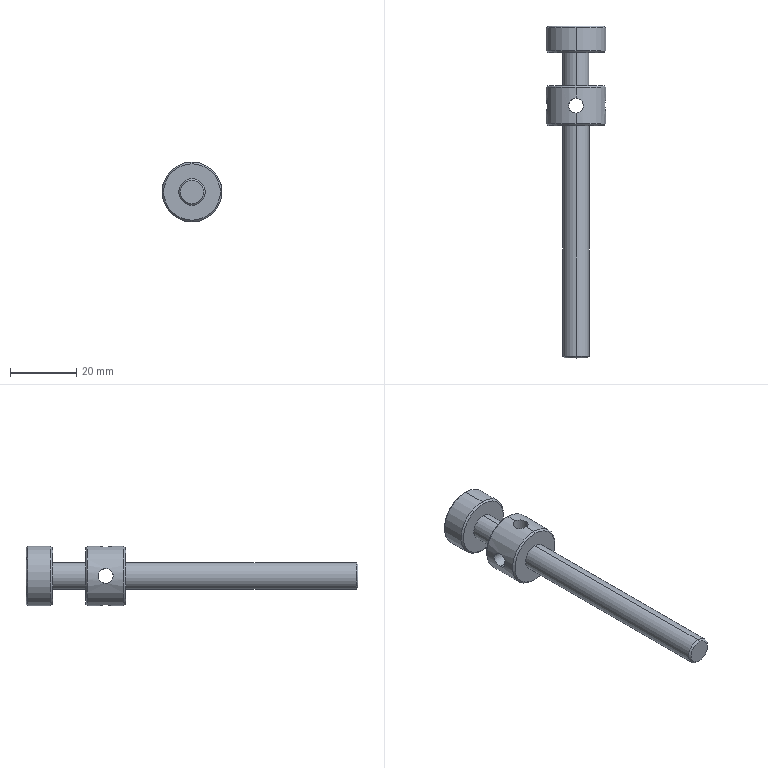Part | SolidWorks | features ICE 4, Chamfer 2, CirPattern 1, Extrusion 1 | 1 solid | 31 faces | box 18 x 100 x 18 mm | volume 8573 mm3 | cylinder 16 | cone 10 | plane 5 | commonest cylinder face diameters 4.5 x8 8 x4 18 x4
STEP:
#1=CARTESIAN_POINT('',(0.,10.,-8.5));
#2=VERTEX_POINT('',#1);
#3=CARTESIAN_POINT('',(0.,10.,8.5));
#4=VERTEX_POINT('',#3);
#5=CARTESIAN_POINT('',(0.,10.,0.));
#6=DIRECTION('',(0.,-1.,0.));
#7=DIRECTION('',(0.,0.,1.));
#8=AXIS2_PLACEMENT_3D('',#5,#6,#7);
#9=CIRCLE('',#8,8.5);
#10=EDGE_CURVE('',#2,#4,#9,.T.);
#11=ORIENTED_EDGE('',*,*,#10,.F.);
#12=CARTESIAN_POINT('',(0.,10.5,-9.));
#13=VERTEX_POINT('',#12);
#14=CARTESIAN_POINT('',(0.,10.5,-9.));
#15=DIRECTION('',(0.,0.7071,-0.7071));
#16=VECTOR('',#15,1000.);
#17=LINE('',#14,#16);
#18=EDGE_CURVE('',#2,#13,#17,.T.);
#19=ORIENTED_EDGE('',*,*,#18,.T.);
#20=CARTESIAN_POINT('',(0.,10.5,9.));
#21=VERTEX_POINT('',#20);
#22=CARTESIAN_POINT('',(0.,10.5,0.));
#23=DIRECTION('',(0.,1.,0.));
#24=DIRECTION('',(0.,0.,1.));
#25=AXIS2_PLACEMENT_3D('',#22,#23,#24);
#26=CIRCLE('',#25,9.);
#27=EDGE_CURVE('',#21,#13,#26,.T.);
#28=ORIENTED_EDGE('',*,*,#27,.F.);
#29=CARTESIAN_POINT('',(0.,10.5,9.));
#30=DIRECTION('',(0.,0.7071,0.7071));
#31=VECTOR('',#30,1000.);
#32=LINE('',#29,#31);
#33=EDGE_CURVE('',#4,#21,#32,.T.);
#34=ORIENTED_EDGE('',*,*,#33,.F.);
#35=EDGE_LOOP('',(#11,#19,#28,#34));
#36=FACE_OUTER_BOUND('',#35,.T.);
#37=CARTESIAN_POINT('',(0.,10.5,0.));
#38=DIRECTION('',(0.,1.,0.));
#39=DIRECTION('',(0.,0.,1.));
#40=AXIS2_PLACEMENT_3D('',#37,#38,#39);
#41=CONICAL_SURFACE('',#40,9.,0.7854);
#42=ADVANCED_FACE('',(#36),#41,.T.);
#43=CARTESIAN_POINT('',(0.,0.,8.5));
#44=VERTEX_POINT('',#43);
#45=CARTESIAN_POINT('',(0.,0.,-8.5));
#46=VERTEX_POINT('',#45);
#47=CARTESIAN_POINT('',(0.,0.,0.));
#48=DIRECTION('',(0.,1.,0.));
#49=DIRECTION('',(0.,0.,-1.));
#50=AXIS2_PLACEMENT_3D('',#47,#48,#49);
#51=CIRCLE('',#50,8.5);
#52=EDGE_CURVE('',#44,#46,#51,.T.);
#53=ORIENTED_EDGE('',*,*,#52,.F.);
#54=CARTESIAN_POINT('',(0.,-0.5,9.));
#55=VERTEX_POINT('',#54);
#56=CARTESIAN_POINT('',(0.,-0.5,9.));
#57=DIRECTION('',(0.,-0.7071,0.7071));
#58=VECTOR('',#57,1000.);
#59=LINE('',#56,#58);
#60=EDGE_CURVE('',#44,#55,#59,.T.);
#61=ORIENTED_EDGE('',*,*,#60,.T.);
#62=CARTESIAN_POINT('',(0.,-0.5,-9.));
#63=VERTEX_POINT('',#62);
#64=CARTESIAN_POINT('',(0.,-0.5,0.));
#65=DIRECTION('',(0.,-1.,0.));
#66=DIRECTION('',(0.,0.,-1.));
#67=AXIS2_PLACEMENT_3D('',#64,#65,#66);
#68=CIRCLE('',#67,9.);
#69=EDGE_CURVE('',#63,#55,#68,.T.);
#70=ORIENTED_EDGE('',*,*,#69,.F.);
#71=CARTESIAN_POINT('',(0.,-0.5,-9.));
#72=DIRECTION('',(0.,-0.7071,-0.7071));
#73=VECTOR('',#72,1000.);
#74=LINE('',#71,#73);
#75=EDGE_CURVE('',#46,#63,#74,.T.);
#76=ORIENTED_EDGE('',*,*,#75,.F.);
#77=EDGE_LOOP('',(#53,#61,#70,#76));
#78=FACE_OUTER_BOUND('',#77,.T.);
#79=CARTESIAN_POINT('',(0.,-0.5,0.));
#80=DIRECTION('',(0.,-1.,0.));
#81=DIRECTION('',(0.,0.,-1.));
#82=AXIS2_PLACEMENT_3D('',#79,#80,#81);
#83=CONICAL_SURFACE('',#82,9.,0.7854);
#84=ADVANCED_FACE('',(#78),#83,.T.);
#85=CARTESIAN_POINT('',(0.,-12.,-8.5));
#86=VERTEX_POINT('',#85);
#87=CARTESIAN_POINT('',(0.,-12.,8.5));
#88=VERTEX_POINT('',#87);
#89=CARTESIAN_POINT('',(0.,-12.,0.));
#90=DIRECTION('',(0.,-1.,0.));
#91=DIRECTION('',(0.,0.,-1.));
#92=AXIS2_PLACEMENT_3D('',#89,#90,#91);
#93=CIRCLE('',#92,8.5);
#94=EDGE_CURVE('',#86,#88,#93,.T.);
#95=ORIENTED_EDGE('',*,*,#94,.F.);
#96=CARTESIAN_POINT('',(0.,-11.5,-9.));
#97=VERTEX_POINT('',#96);
#98=CARTESIAN_POINT('',(0.,-12.,-8.5));
#99=DIRECTION('',(0.,0.7071,-0.7071));
#100=VECTOR('',#99,1000.);
#101=LINE('',#98,#100);
#102=EDGE_CURVE('',#86,#97,#101,.T.);
#103=ORIENTED_EDGE('',*,*,#102,.T.);
#104=CARTESIAN_POINT('',(0.,-11.5,9.));
#105=VERTEX_POINT('',#104);
#106=CARTESIAN_POINT('',(0.,-11.5,0.));
#107=DIRECTION('',(0.,1.,0.));
#108=DIRECTION('',(0.,0.,-1.));
#109=AXIS2_PLACEMENT_3D('',#106,#107,#108);
#110=CIRCLE('',#109,9.);
#111=EDGE_CURVE('',#105,#97,#110,.T.);
#112=ORIENTED_EDGE('',*,*,#111,.F.);
#113=CARTESIAN_POINT('',(0.,-12.,8.5));
#114=DIRECTION('',(0.,0.7071,0.7071));
#115=VECTOR('',#114,1000.);
#116=LINE('',#113,#115);
#117=EDGE_CURVE('',#88,#105,#116,.T.);
#118=ORIENTED_EDGE('',*,*,#117,.F.);
#119=EDGE_LOOP('',(#95,#103,#112,#118));
#120=FACE_OUTER_BOUND('',#119,.T.);
#121=CARTESIAN_POINT('',(0.,-12.,0.));
#122=DIRECTION('',(0.,1.,0.));
#123=DIRECTION('',(0.,0.,1.));
#124=AXIS2_PLACEMENT_3D('',#121,#122,#123);
#125=CONICAL_SURFACE('',#124,8.5,0.7854);
#126=ADVANCED_FACE('',(#120),#125,.T.);
#127=CARTESIAN_POINT('',(0.,18.,8.5));
#128=VERTEX_POINT('',#127);
#129=CARTESIAN_POINT('',(0.,18.,-8.5));
#130=VERTEX_POINT('',#129);
#131=CARTESIAN_POINT('',(0.,18.,0.));
#132=DIRECTION('',(0.,1.,0.));
#133=DIRECTION('',(0.,0.,1.));
#134=AXIS2_PLACEMENT_3D('',#131,#132,#133);
#135=CIRCLE('',#134,8.5);
#136=EDGE_CURVE('',#128,#130,#135,.T.);
#137=ORIENTED_EDGE('',*,*,#136,.F.);
#138=CARTESIAN_POINT('',(0.,17.5,9.));
#139=VERTEX_POINT('',#138);
#140=CARTESIAN_POINT('',(0.,18.,8.5));
#141=DIRECTION('',(0.,-0.7071,0.7071));
#142=VECTOR('',#141,1000.);
#143=LINE('',#140,#142);
#144=EDGE_CURVE('',#128,#139,#143,.T.);
#145=ORIENTED_EDGE('',*,*,#144,.T.);
#146=CARTESIAN_POINT('',(0.,17.5,-9.));
#147=VERTEX_POINT('',#146);
#148=CARTESIAN_POINT('',(0.,17.5,0.));
#149=DIRECTION('',(0.,-1.,0.));
#150=DIRECTION('',(0.,0.,1.));
#151=AXIS2_PLACEMENT_3D('',#148,#149,#150);
#152=CIRCLE('',#151,9.);
#153=EDGE_CURVE('',#147,#139,#152,.T.);
#154=ORIENTED_EDGE('',*,*,#153,.F.);
#155=CARTESIAN_POINT('',(0.,18.,-8.5));
#156=DIRECTION('',(0.,-0.7071,-0.7071));
#157=VECTOR('',#156,1000.);
#158=LINE('',#155,#157);
#159=EDGE_CURVE('',#130,#147,#158,.T.);
#160=ORIENTED_EDGE('',*,*,#159,.F.);
#161=EDGE_LOOP('',(#137,#145,#154,#160));
#162=FACE_OUTER_BOUND('',#161,.T.);
#163=CARTESIAN_POINT('',(0.,18.,0.));
#164=DIRECTION('',(0.,-1.,0.));
#165=DIRECTION('',(0.,0.,-1.));
#166=AXIS2_PLACEMENT_3D('',#163,#164,#165);
#167=CONICAL_SURFACE('',#166,8.5,0.7854);
#168=ADVANCED_FACE('',(#162),#167,.T.);
#169=CARTESIAN_POINT('',(2.25,-6.,8.714));
#170=VERTEX_POINT('',#169);
#171=CARTESIAN_POINT('',(0.,-8.25,9.));
#172=VERTEX_POINT('',#171);
#173=CARTESIAN_POINT('',(2.25,-6.,8.714));
#174=CARTESIAN_POINT('',(2.25,-6.148,8.714));
#175=CARTESIAN_POINT('',(2.235,-6.295,8.718));
#176=CARTESIAN_POINT('',(2.178,-6.584,8.733));
#177=CARTESIAN_POINT('',(2.134,-6.727,8.743));
#178=CARTESIAN_POINT('',(1.965,-7.134,8.784));
#179=CARTESIAN_POINT('',(1.798,-7.384,8.821));
#180=CARTESIAN_POINT('',(1.385,-7.797,8.895));
#181=CARTESIAN_POINT('',(1.136,-7.964,8.932));
#182=CARTESIAN_POINT('',(0.7295,-8.133,8.971));
#183=CARTESIAN_POINT('',(0.5862,-8.177,8.982));
#184=CARTESIAN_POINT('',(0.2963,-8.235,8.996));
#185=CARTESIAN_POINT('',(0.1492,-8.25,9.));
#186=CARTESIAN_POINT('',(0.,-8.25,9.));
#187=B_SPLINE_CURVE_WITH_KNOTS('',3,(#173,#174,#175,#176,#177,#178,#179,#180,#181,#182,#183,#184,#185,#186),.UNSPECIFIED.,.F.,.F.,(4,2,2,2,2,2,4),(0.01059,0.01103,0.01148,0.01236,0.01324,0.01368,0.01412),.UNSPECIFIED.);
#188=EDGE_CURVE('',#170,#172,#187,.T.);
#189=ORIENTED_EDGE('',*,*,#188,.F.);
#190=CARTESIAN_POINT('',(2.25,-6.,2.25));
#191=VERTEX_POINT('',#190);
#192=CARTESIAN_POINT('',(2.25,-6.,10.));
#193=DIRECTION('',(0.,0.,-1.));
#194=VECTOR('',#193,1000.);
#195=LINE('',#192,#194);
#196=EDGE_CURVE('',#170,#191,#195,.T.);
#197=ORIENTED_EDGE('',*,*,#196,.T.);
#198=CARTESIAN_POINT('',(0.,-8.25,0.));
#199=VERTEX_POINT('',#198);
#200=CARTESIAN_POINT('',(0.,-8.25,0.));
#201=CARTESIAN_POINT('',(1.318,-8.25,1.318));
#202=CARTESIAN_POINT('',(2.25,-7.318,2.25));
#203=CARTESIAN_POINT('',(2.25,-6.,2.25));
#204=(BOUNDED_CURVE()B_SPLINE_CURVE(3,(#200,#201,#202,#203),.UNSPECIFIED.,.F.,.T.)B_SPLINE_CURVE_WITH_KNOTS((4,4),(1.571,3.142),.UNSPECIFIED.)CURVE()GEOMETRIC_REPRESENTATION_ITEM()RATIONAL_B_SPLINE_CURVE((1.,0.8047,0.8047,1.))REPRESENTATION_ITEM(''));
#205=EDGE_CURVE('',#199,#191,#204,.T.);
#206=ORIENTED_EDGE('',*,*,#205,.F.);
#207=CARTESIAN_POINT('',(-2.25,-6.,2.25));
#208=VERTEX_POINT('',#207);
#209=CARTESIAN_POINT('',(0.,-8.25,0.));
#210=CARTESIAN_POINT('',(-1.318,-8.25,1.318));
#211=CARTESIAN_POINT('',(-2.25,-7.318,2.25));
#212=CARTESIAN_POINT('',(-2.25,-6.,2.25));
#213=(BOUNDED_CURVE()B_SPLINE_CURVE(3,(#209,#210,#211,#212),.UNSPECIFIED.,.F.,.T.)B_SPLINE_CURVE_WITH_KNOTS((4,4),(1.571,3.142),.UNSPECIFIED.)CURVE()GEOMETRIC_REPRESENTATION_ITEM()RATIONAL_B_SPLINE_CURVE((1.,0.8047,0.8047,1.))REPRESENTATION_ITEM(''));
#214=EDGE_CURVE('',#199,#208,#213,.T.);
#215=ORIENTED_EDGE('',*,*,#214,.T.);
#216=CARTESIAN_POINT('',(-2.25,-6.,8.714));
#217=VERTEX_POINT('',#216);
#218=CARTESIAN_POINT('',(-2.25,-6.,10.));
#219=DIRECTION('',(0.,0.,-1.));
#220=VECTOR('',#219,1000.);
#221=LINE('',#218,#220);
#222=EDGE_CURVE('',#217,#208,#221,.T.);
#223=ORIENTED_EDGE('',*,*,#222,.F.);
#224=CARTESIAN_POINT('',(0.,-8.25,9.));
#225=CARTESIAN_POINT('',(-0.1493,-8.25,9.));
#226=CARTESIAN_POINT('',(-0.2961,-8.235,8.996));
#227=CARTESIAN_POINT('',(-0.5845,-8.178,8.982));
#228=CARTESIAN_POINT('',(-0.7278,-8.134,8.972));
#229=CARTESIAN_POINT('',(-1.,-8.021,8.945));
#230=CARTESIAN_POINT('',(-1.129,-7.952,8.93));
#231=CARTESIAN_POINT('',(-1.373,-7.788,8.895));
#232=CARTESIAN_POINT('',(-1.488,-7.694,8.877));
#233=CARTESIAN_POINT('',(-1.798,-7.383,8.821));
#234=CARTESIAN_POINT('',(-1.966,-7.133,8.783));
#235=CARTESIAN_POINT('',(-2.134,-6.727,8.743));
#236=CARTESIAN_POINT('',(-2.178,-6.585,8.733));
#237=CARTESIAN_POINT('',(-2.236,-6.294,8.718));
#238=CARTESIAN_POINT('',(-2.25,-6.147,8.714));
#239=CARTESIAN_POINT('',(-2.25,-6.,8.714));
#240=B_SPLINE_CURVE_WITH_KNOTS('',3,(#224,#225,#226,#227,#228,#229,#230,#231,#232,#233,#234,#235,#236,#237,#238,#239),.UNSPECIFIED.,.F.,.F.,(4,2,2,2,2,2,2,4),(0.,0.0004415,0.0008831,0.001325,0.001766,0.002649,0.003091,0.003532),.UNSPECIFIED.);
#241=EDGE_CURVE('',#172,#217,#240,.T.);
#242=ORIENTED_EDGE('',*,*,#241,.F.);
#243=EDGE_LOOP('',(#189,#197,#206,#215,#223,#242));
#244=FACE_OUTER_BOUND('',#243,.T.);
#245=CARTESIAN_POINT('',(0.,-6.,10.));
#246=DIRECTION('',(0.,0.,-1.));
#247=DIRECTION('',(-1.,0.,0.));
#248=AXIS2_PLACEMENT_3D('',#245,#246,#247);
#249=CYLINDRICAL_SURFACE('',#248,2.25);
#250=ADVANCED_FACE('',(#244),#249,.F.);
#251=CARTESIAN_POINT('',(-2.25,-6.,-2.25));
#252=VERTEX_POINT('',#251);
#253=CARTESIAN_POINT('',(-2.25,-6.,-2.25));
#254=CARTESIAN_POINT('',(-2.25,-7.318,-2.25));
#255=CARTESIAN_POINT('',(-1.318,-8.25,-1.318));
#256=CARTESIAN_POINT('',(0.,-8.25,0.));
#257=(BOUNDED_CURVE()B_SPLINE_CURVE(3,(#253,#254,#255,#256),.UNSPECIFIED.,.F.,.T.)B_SPLINE_CURVE_WITH_KNOTS((4,4),(3.142,4.712),.UNSPECIFIED.)CURVE()GEOMETRIC_REPRESENTATION_ITEM()RATIONAL_B_SPLINE_CURVE((1.,0.8047,0.8047,1.))REPRESENTATION_ITEM(''));
#258=EDGE_CURVE('',#252,#199,#257,.T.);
#259=ORIENTED_EDGE('',*,*,#258,.F.);
#260=CARTESIAN_POINT('',(-8.714,-6.,-2.25));
#261=VERTEX_POINT('',#260);
#262=CARTESIAN_POINT('',(10.,-6.,-2.25));
#263=DIRECTION('',(-1.,0.,0.));
#264=VECTOR('',#263,1000.);
#265=LINE('',#262,#264);
#266=EDGE_CURVE('',#252,#261,#265,.T.);
#267=ORIENTED_EDGE('',*,*,#266,.T.);
#268=CARTESIAN_POINT('',(-8.714,-6.,2.25));
#269=VERTEX_POINT('',#268);
#270=CARTESIAN_POINT('',(-8.714,-6.,2.25));
#271=CARTESIAN_POINT('',(-8.714,-6.149,2.25));
#272=CARTESIAN_POINT('',(-8.718,-6.296,2.235));
#273=CARTESIAN_POINT('',(-8.733,-6.584,2.178));
#274=CARTESIAN_POINT('',(-8.743,-6.728,2.134));
#275=CARTESIAN_POINT('',(-8.77,-7.,2.021));
#276=CARTESIAN_POINT('',(-8.786,-7.129,1.952));
#277=CARTESIAN_POINT('',(-8.821,-7.373,1.789));
#278=CARTESIAN_POINT('',(-8.84,-7.488,1.694));
#279=CARTESIAN_POINT('',(-8.895,-7.798,1.384));
#280=CARTESIAN_POINT('',(-8.932,-7.965,1.134));
#281=CARTESIAN_POINT('',(-8.972,-8.134,0.728));
#282=CARTESIAN_POINT('',(-8.982,-8.178,0.5855));
#283=CARTESIAN_POINT('',(-8.996,-8.236,0.2947));
#284=CARTESIAN_POINT('',(-9.,-8.25,0.1483));
#285=CARTESIAN_POINT('',(-9.,-8.25,-0.1465));
#286=CARTESIAN_POINT('',(-8.996,-8.235,-0.2963));
#287=CARTESIAN_POINT('',(-8.982,-8.178,-0.5854));
#288=CARTESIAN_POINT('',(-8.972,-8.135,-0.7259));
#289=CARTESIAN_POINT('',(-8.932,-7.965,-1.136));
#290=CARTESIAN_POINT('',(-8.896,-7.799,-1.383));
#291=CARTESIAN_POINT('',(-8.839,-7.486,-1.696));
#292=CARTESIAN_POINT('',(-8.821,-7.373,-1.788));
#293=CARTESIAN_POINT('',(-8.786,-7.13,-1.951));
#294=CARTESIAN_POINT('',(-8.77,-6.998,-2.022));
#295=CARTESIAN_POINT('',(-8.743,-6.727,-2.135));
#296=CARTESIAN_POINT('',(-8.733,-6.586,-2.177));
#297=CARTESIAN_POINT('',(-8.718,-6.297,-2.235));
#298=CARTESIAN_POINT('',(-8.714,-6.147,-2.25));
#299=CARTESIAN_POINT('',(-8.714,-6.,-2.25));
#300=B_SPLINE_CURVE_WITH_KNOTS('',3,(#270,#271,#272,#273,#274,#275,#276,#277,#278,#279,#280,#281,#282,#283,#284,#285,#286,#287,#288,#289,#290,#291,#292,#293,#294,#295,#296,#297,#298,#299),.UNSPECIFIED.,.F.,.F.,(4,2,2,2,2,2,2,2,2,2,2,2,2,2,4),(0.,0.0004414,0.0008828,0.001324,0.001766,0.002648,0.00309,0.003531,0.003973,0.004414,0.005297,0.005738,0.00618,0.006621,0.007063),.UNSPECIFIED.);
#301=EDGE_CURVE('',#269,#261,#300,.T.);
#302=ORIENTED_EDGE('',*,*,#301,.F.);
#303=CARTESIAN_POINT('',(10.,-6.,2.25));
#304=DIRECTION('',(-1.,0.,0.));
#305=VECTOR('',#304,1000.);
#306=LINE('',#303,#305);
#307=EDGE_CURVE('',#208,#269,#306,.T.);
#308=ORIENTED_EDGE('',*,*,#307,.F.);
#309=ORIENTED_EDGE('',*,*,#214,.F.);
#310=EDGE_LOOP('',(#259,#267,#302,#308,#309));
#311=FACE_OUTER_BOUND('',#310,.T.);
#312=CARTESIAN_POINT('',(10.,-6.,0.));
#313=DIRECTION('',(-1.,0.,0.));
#314=DIRECTION('',(0.,0.,1.));
#315=AXIS2_PLACEMENT_3D('',#312,#313,#314);
#316=CYLINDRICAL_SURFACE('',#315,2.25);
#317=ADVANCED_FACE('',(#311),#316,.F.);
#318=CARTESIAN_POINT('',(8.714,-6.,-2.25));
#319=VERTEX_POINT('',#318);
#320=CARTESIAN_POINT('',(8.714,-6.,2.25));
#321=VERTEX_POINT('',#320);
#322=CARTESIAN_POINT('',(8.714,-6.,-2.25));
#323=CARTESIAN_POINT('',(8.714,-6.294,-2.25));
#324=CARTESIAN_POINT('',(8.73,-6.591,-2.191));
#325=CARTESIAN_POINT('',(8.77,-6.998,-2.022));
#326=CARTESIAN_POINT('',(8.786,-7.129,-1.952));
#327=CARTESIAN_POINT('',(8.821,-7.374,-1.788));
#328=CARTESIAN_POINT('',(8.839,-7.486,-1.695));
#329=CARTESIAN_POINT('',(8.877,-7.694,-1.488));
#330=CARTESIAN_POINT('',(8.896,-7.789,-1.373));
#331=CARTESIAN_POINT('',(8.93,-7.951,-1.13));
#332=CARTESIAN_POINT('',(8.945,-8.021,-1.001));
#333=CARTESIAN_POINT('',(8.985,-8.191,-0.5904));
#334=CARTESIAN_POINT('',(9.,-8.25,-0.2975));
#335=CARTESIAN_POINT('',(9.,-8.25,0.1477));
#336=CARTESIAN_POINT('',(8.996,-8.236,0.2941));
#337=CARTESIAN_POINT('',(8.982,-8.178,0.5832));
#338=CARTESIAN_POINT('',(8.972,-8.134,0.7268));
#339=CARTESIAN_POINT('',(8.932,-7.965,1.134));
#340=CARTESIAN_POINT('',(8.895,-7.798,1.384));
#341=CARTESIAN_POINT('',(8.821,-7.385,1.797));
#342=CARTESIAN_POINT('',(8.784,-7.136,1.964));
#343=CARTESIAN_POINT('',(8.744,-6.73,2.133));
#344=CARTESIAN_POINT('',(8.733,-6.586,2.177));
#345=CARTESIAN_POINT('',(8.718,-6.296,2.235));
#346=CARTESIAN_POINT('',(8.714,-6.149,2.25));
#347=CARTESIAN_POINT('',(8.714,-6.,2.25));
#348=B_SPLINE_CURVE_WITH_KNOTS('',3,(#322,#323,#324,#325,#326,#327,#328,#329,#330,#331,#332,#333,#334,#335,#336,#337,#338,#339,#340,#341,#342,#343,#344,#345,#346,#347),.UNSPECIFIED.,.F.,.F.,(4,2,2,2,2,2,2,2,2,2,2,2,4),(0.007063,0.007945,0.008386,0.008828,0.009269,0.00971,0.01059,0.01103,0.01148,0.01236,0.01324,0.01368,0.01412),.UNSPECIFIED.);
#349=EDGE_CURVE('',#319,#321,#348,.T.);
#350=ORIENTED_EDGE('',*,*,#349,.F.);
#351=CARTESIAN_POINT('',(2.25,-6.,-2.25));
#352=VERTEX_POINT('',#351);
#353=CARTESIAN_POINT('',(10.,-6.,-2.25));
#354=DIRECTION('',(-1.,0.,0.));
#355=VECTOR('',#354,1000.);
#356=LINE('',#353,#355);
#357=EDGE_CURVE('',#319,#352,#356,.T.);
#358=ORIENTED_EDGE('',*,*,#357,.T.);
#359=CARTESIAN_POINT('',(0.,-8.25,0.));
#360=CARTESIAN_POINT('',(1.318,-8.25,-1.318));
#361=CARTESIAN_POINT('',(2.25,-7.318,-2.25));
#362=CARTESIAN_POINT('',(2.25,-6.,-2.25));
#363=(BOUNDED_CURVE()B_SPLINE_CURVE(3,(#359,#360,#361,#362),.UNSPECIFIED.,.F.,.T.)B_SPLINE_CURVE_WITH_KNOTS((4,4),(1.571,3.142),.UNSPECIFIED.)CURVE()GEOMETRIC_REPRESENTATION_ITEM()RATIONAL_B_SPLINE_CURVE((1.,0.8047,0.8047,1.))REPRESENTATION_ITEM(''));
#364=EDGE_CURVE('',#199,#352,#363,.T.);
#365=ORIENTED_EDGE('',*,*,#364,.F.);
#366=ORIENTED_EDGE('',*,*,#205,.T.);
#367=CARTESIAN_POINT('',(10.,-6.,2.25));
#368=DIRECTION('',(-1.,0.,0.));
#369=VECTOR('',#368,1000.);
#370=LINE('',#367,#369);
#371=EDGE_CURVE('',#321,#191,#370,.T.);
#372=ORIENTED_EDGE('',*,*,#371,.F.);
#373=EDGE_LOOP('',(#350,#358,#365,#366,#372));
#374=FACE_OUTER_BOUND('',#373,.T.);
#375=CARTESIAN_POINT('',(10.,-6.,0.));
#376=DIRECTION('',(-1.,0.,0.));
#377=DIRECTION('',(0.,0.,1.));
#378=AXIS2_PLACEMENT_3D('',#375,#376,#377);
#379=CYLINDRICAL_SURFACE('',#378,2.25);
#380=ADVANCED_FACE('',(#374),#379,.F.);
#381=CARTESIAN_POINT('',(-2.25,-6.,-8.714));
#382=VERTEX_POINT('',#381);
#383=CARTESIAN_POINT('',(0.,-8.25,-9.));
#384=VERTEX_POINT('',#383);
#385=CARTESIAN_POINT('',(-2.25,-6.,-8.714));
#386=CARTESIAN_POINT('',(-2.25,-6.294,-8.714));
#387=CARTESIAN_POINT('',(-2.191,-6.592,-8.73));
#388=CARTESIAN_POINT('',(-2.022,-6.998,-8.77));
#389=CARTESIAN_POINT('',(-1.951,-7.13,-8.786));
#390=CARTESIAN_POINT('',(-1.788,-7.374,-8.821));
#391=CARTESIAN_POINT('',(-1.695,-7.487,-8.84));
#392=CARTESIAN_POINT('',(-1.488,-7.694,-8.877));
#393=CARTESIAN_POINT('',(-1.373,-7.789,-8.896));
#394=CARTESIAN_POINT('',(-1.13,-7.951,-8.93));
#395=CARTESIAN_POINT('',(-1.001,-8.021,-8.945));
#396=CARTESIAN_POINT('',(-0.5898,-8.191,-8.985));
#397=CARTESIAN_POINT('',(-0.2968,-8.25,-9.));
#398=CARTESIAN_POINT('',(0.,-8.25,-9.));
#399=B_SPLINE_CURVE_WITH_KNOTS('',3,(#385,#386,#387,#388,#389,#390,#391,#392,#393,#394,#395,#396,#397,#398),.UNSPECIFIED.,.F.,.F.,(4,2,2,2,2,2,4),(0.007063,0.007945,0.008387,0.008828,0.009269,0.009711,0.01059),.UNSPECIFIED.);
#400=EDGE_CURVE('',#382,#384,#399,.T.);
#401=ORIENTED_EDGE('',*,*,#400,.F.);
#402=CARTESIAN_POINT('',(-2.25,-6.,-10.));
#403=DIRECTION('',(0.,0.,1.));
#404=VECTOR('',#403,1000.);
#405=LINE('',#402,#404);
#406=EDGE_CURVE('',#382,#252,#405,.T.);
#407=ORIENTED_EDGE('',*,*,#406,.T.);
#408=ORIENTED_EDGE('',*,*,#258,.T.);
#409=ORIENTED_EDGE('',*,*,#364,.T.);
#410=CARTESIAN_POINT('',(2.25,-6.,-8.714));
#411=VERTEX_POINT('',#410);
#412=CARTESIAN_POINT('',(2.25,-6.,-10.));
#413=DIRECTION('',(0.,0.,1.));
#414=VECTOR('',#413,1000.);
#415=LINE('',#412,#414);
#416=EDGE_CURVE('',#411,#352,#415,.T.);
#417=ORIENTED_EDGE('',*,*,#416,.F.);
#418=CARTESIAN_POINT('',(0.,-8.25,-9.));
#419=CARTESIAN_POINT('',(0.1484,-8.25,-9.));
#420=CARTESIAN_POINT('',(0.2948,-8.235,-8.996));
#421=CARTESIAN_POINT('',(0.5837,-8.178,-8.982));
#422=CARTESIAN_POINT('',(0.7273,-8.134,-8.972));
#423=CARTESIAN_POINT('',(1.134,-7.965,-8.932));
#424=CARTESIAN_POINT('',(1.384,-7.798,-8.895));
#425=CARTESIAN_POINT('',(1.797,-7.385,-8.821));
#426=CARTESIAN_POINT('',(1.964,-7.136,-8.784));
#427=CARTESIAN_POINT('',(2.134,-6.729,-8.744));
#428=CARTESIAN_POINT('',(2.177,-6.586,-8.733));
#429=CARTESIAN_POINT('',(2.235,-6.296,-8.718));
#430=CARTESIAN_POINT('',(2.25,-6.149,-8.714));
#431=CARTESIAN_POINT('',(2.25,-6.,-8.714));
#432=B_SPLINE_CURVE_WITH_KNOTS('',3,(#418,#419,#420,#421,#422,#423,#424,#425,#426,#427,#428,#429,#430,#431),.UNSPECIFIED.,.F.,.F.,(4,2,2,2,2,2,4),(0.01059,0.01103,0.01148,0.01236,0.01324,0.01368,0.01412),.UNSPECIFIED.);
#433=EDGE_CURVE('',#384,#411,#432,.T.);
#434=ORIENTED_EDGE('',*,*,#433,.F.);
#435=EDGE_LOOP('',(#401,#407,#408,#409,#417,#434));
#436=FACE_OUTER_BOUND('',#435,.T.);
#437=CARTESIAN_POINT('',(0.,-6.,-10.));
#438=DIRECTION('',(0.,0.,1.));
#439=DIRECTION('',(1.,0.,0.));
#440=AXIS2_PLACEMENT_3D('',#437,#438,#439);
#441=CYLINDRICAL_SURFACE('',#440,2.25);
#442=ADVANCED_FACE('',(#436),#441,.F.);
#443=CARTESIAN_POINT('',(0.,-82.,-3.5));
#444=VERTEX_POINT('',#443);
#445=CARTESIAN_POINT('',(0.,-82.,3.5));
#446=VERTEX_POINT('',#445);
#447=CARTESIAN_POINT('',(0.,-82.,0.));
#448=DIRECTION('',(0.,-1.,0.));
#449=DIRECTION('',(0.,0.,-1.));
#450=AXIS2_PLACEMENT_3D('',#447,#448,#449);
#451=CIRCLE('',#450,3.5);
#452=EDGE_CURVE('',#444,#446,#451,.T.);
#453=ORIENTED_EDGE('',*,*,#452,.F.);
#454=CARTESIAN_POINT('',(0.,-81.5,-4.));
#455=VERTEX_POINT('',#454);
#456=CARTESIAN_POINT('',(0.,-82.,-3.5));
#457=DIRECTION('',(0.,0.7071,-0.7071));
#458=VECTOR('',#457,1000.);
#459=LINE('',#456,#458);
#460=EDGE_CURVE('',#444,#455,#459,.T.);
#461=ORIENTED_EDGE('',*,*,#460,.T.);
#462=CARTESIAN_POINT('',(0.,-81.5,4.));
#463=VERTEX_POINT('',#462);
#464=CARTESIAN_POINT('',(0.,-81.5,0.));
#465=DIRECTION('',(0.,1.,0.));
#466=DIRECTION('',(0.,0.,-1.));
#467=AXIS2_PLACEMENT_3D('',#464,#465,#466);
#468=CIRCLE('',#467,4.);
#469=EDGE_CURVE('',#463,#455,#468,.T.);
#470=ORIENTED_EDGE('',*,*,#469,.F.);
#471=CARTESIAN_POINT('',(0.,-82.,3.5));
#472=DIRECTION('',(0.,0.7071,0.7071));
#473=VECTOR('',#472,1000.);
#474=LINE('',#471,#473);
#475=EDGE_CURVE('',#446,#463,#474,.T.);
#476=ORIENTED_EDGE('',*,*,#475,.F.);
#477=EDGE_LOOP('',(#453,#461,#470,#476));
#478=FACE_OUTER_BOUND('',#477,.T.);
#479=CARTESIAN_POINT('',(0.,-82.,0.));
#480=DIRECTION('',(0.,1.,0.));
#481=DIRECTION('',(0.,0.,1.));
#482=AXIS2_PLACEMENT_3D('',#479,#480,#481);
#483=CONICAL_SURFACE('',#482,3.5,0.7854);
#484=ADVANCED_FACE('',(#478),#483,.T.);
#485=ORIENTED_EDGE('',*,*,#469,.T.);
#486=CARTESIAN_POINT('',(0.,-12.,-4.));
#487=VERTEX_POINT('',#486);
#488=CARTESIAN_POINT('',(0.,-82.,-4.));
#489=DIRECTION('',(0.,1.,0.));
#490=VECTOR('',#489,1000.);
#491=LINE('',#488,#490);
#492=EDGE_CURVE('',#455,#487,#491,.T.);
#493=ORIENTED_EDGE('',*,*,#492,.T.);
#494=CARTESIAN_POINT('',(0.,-12.,4.));
#495=VERTEX_POINT('',#494);
#496=CARTESIAN_POINT('',(0.,-12.,0.));
#497=DIRECTION('',(0.,-1.,0.));
#498=DIRECTION('',(0.,0.,-1.));
#499=AXIS2_PLACEMENT_3D('',#496,#497,#498);
#500=CIRCLE('',#499,4.);
#501=EDGE_CURVE('',#487,#495,#500,.T.);
#502=ORIENTED_EDGE('',*,*,#501,.T.);
#503=CARTESIAN_POINT('',(0.,-82.,4.));
#504=DIRECTION('',(0.,1.,0.));
#505=VECTOR('',#504,1000.);
#506=LINE('',#503,#505);
#507=EDGE_CURVE('',#463,#495,#506,.T.);
#508=ORIENTED_EDGE('',*,*,#507,.F.);
#509=EDGE_LOOP('',(#485,#493,#502,#508));
#510=FACE_OUTER_BOUND('',#509,.T.);
#511=CARTESIAN_POINT('',(0.,-82.,0.));
#512=DIRECTION('',(0.,1.,0.));
#513=DIRECTION('',(0.,0.,1.));
#514=AXIS2_PLACEMENT_3D('',#511,#512,#513);
#515=CYLINDRICAL_SURFACE('',#514,4.);
#516=ADVANCED_FACE('',(#510),#515,.T.);
#517=CARTESIAN_POINT('',(8.714,-6.,2.25));
#518=CARTESIAN_POINT('',(8.714,-5.851,2.25));
#519=CARTESIAN_POINT('',(8.718,-5.704,2.235));
#520=CARTESIAN_POINT('',(8.733,-5.416,2.178));
#521=CARTESIAN_POINT('',(8.743,-5.272,2.134));
#522=CARTESIAN_POINT('',(8.77,-5.,2.021));
#523=CARTESIAN_POINT('',(8.786,-4.871,1.952));
#524=CARTESIAN_POINT('',(8.821,-4.627,1.789));
#525=CARTESIAN_POINT('',(8.84,-4.512,1.694));
#526=CARTESIAN_POINT('',(8.895,-4.202,1.384));
#527=CARTESIAN_POINT('',(8.932,-4.035,1.134));
#528=CARTESIAN_POINT('',(8.972,-3.866,0.728));
#529=CARTESIAN_POINT('',(8.982,-3.822,0.5855));
#530=CARTESIAN_POINT('',(8.996,-3.764,0.2947));
#531=CARTESIAN_POINT('',(9.,-3.75,0.1483));
#532=CARTESIAN_POINT('',(9.,-3.75,-0.1465));
#533=CARTESIAN_POINT('',(8.996,-3.765,-0.2963));
#534=CARTESIAN_POINT('',(8.982,-3.822,-0.5854));
#535=CARTESIAN_POINT('',(8.972,-3.865,-0.7259));
#536=CARTESIAN_POINT('',(8.932,-4.035,-1.136));
#537=CARTESIAN_POINT('',(8.896,-4.201,-1.383));
#538=CARTESIAN_POINT('',(8.839,-4.514,-1.696));
#539=CARTESIAN_POINT('',(8.821,-4.627,-1.788));
#540=CARTESIAN_POINT('',(8.786,-4.87,-1.951));
#541=CARTESIAN_POINT('',(8.77,-5.002,-2.022));
#542=CARTESIAN_POINT('',(8.743,-5.273,-2.135));
#543=CARTESIAN_POINT('',(8.733,-5.414,-2.177));
#544=CARTESIAN_POINT('',(8.718,-5.703,-2.235));
#545=CARTESIAN_POINT('',(8.714,-5.853,-2.25));
#546=CARTESIAN_POINT('',(8.714,-6.,-2.25));
#547=B_SPLINE_CURVE_WITH_KNOTS('',3,(#517,#518,#519,#520,#521,#522,#523,#524,#525,#526,#527,#528,#529,#530,#531,#532,#533,#534,#535,#536,#537,#538,#539,#540,#541,#542,#543,#544,#545,#546),.UNSPECIFIED.,.F.,.F.,(4,2,2,2,2,2,2,2,2,2,2,2,2,2,4),(0.,0.0004414,0.0008828,0.001324,0.001766,0.002648,0.00309,0.003531,0.003973,0.004414,0.005297,0.005738,0.00618,0.006621,0.007063),.UNSPECIFIED.);
#548=EDGE_CURVE('',#321,#319,#547,.T.);
#549=ORIENTED_EDGE('',*,*,#548,.T.);
#550=ORIENTED_EDGE('',*,*,#349,.T.);
#551=EDGE_LOOP('',(#549,#550));
#552=FACE_BOUND('',#551,.T.);
#553=ORIENTED_EDGE('',*,*,#111,.T.);
#554=CARTESIAN_POINT('',(0.,-12.,-9.));
#555=DIRECTION('',(0.,1.,0.));
#556=VECTOR('',#555,1000.);
#557=LINE('',#554,#556);
#558=EDGE_CURVE('',#97,#384,#557,.T.);
#559=ORIENTED_EDGE('',*,*,#558,.T.);
#560=ORIENTED_EDGE('',*,*,#433,.T.);
#561=CARTESIAN_POINT('',(0.,-3.75,-9.));
#562=VERTEX_POINT('',#561);
#563=CARTESIAN_POINT('',(2.25,-6.,-8.714));
#564=CARTESIAN_POINT('',(2.25,-5.851,-8.714));
#565=CARTESIAN_POINT('',(2.235,-5.704,-8.718));
#566=CARTESIAN_POINT('',(2.178,-5.415,-8.733));
#567=CARTESIAN_POINT('',(2.134,-5.272,-8.744));
#568=CARTESIAN_POINT('',(2.021,-5.,-8.77));
#569=CARTESIAN_POINT('',(1.952,-4.871,-8.786));
#570=CARTESIAN_POINT('',(1.788,-4.627,-8.821));
#571=CARTESIAN_POINT('',(1.694,-4.512,-8.84));
#572=CARTESIAN_POINT('',(1.384,-4.202,-8.896));
#573=CARTESIAN_POINT('',(1.133,-4.034,-8.933));
#574=CARTESIAN_POINT('',(0.7273,-3.866,-8.972));
#575=CARTESIAN_POINT('',(0.5848,-3.822,-8.982));
#576=CARTESIAN_POINT('',(0.2939,-3.764,-8.996));
#577=CARTESIAN_POINT('',(0.1475,-3.75,-9.));
#578=CARTESIAN_POINT('',(0.,-3.75,-9.));
#579=B_SPLINE_CURVE_WITH_KNOTS('',3,(#563,#564,#565,#566,#567,#568,#569,#570,#571,#572,#573,#574,#575,#576,#577,#578),.UNSPECIFIED.,.F.,.F.,(4,2,2,2,2,2,2,4),(0.,0.0004415,0.0008831,0.001325,0.001766,0.002649,0.003091,0.003532),.UNSPECIFIED.);
#580=EDGE_CURVE('',#411,#562,#579,.T.);
#581=ORIENTED_EDGE('',*,*,#580,.T.);
#582=CARTESIAN_POINT('',(0.,-12.,-9.));
#583=DIRECTION('',(0.,1.,0.));
#584=VECTOR('',#583,1000.);
#585=LINE('',#582,#584);
#586=EDGE_CURVE('',#562,#63,#585,.T.);
#587=ORIENTED_EDGE('',*,*,#586,.T.);
#588=ORIENTED_EDGE('',*,*,#69,.T.);
#589=CARTESIAN_POINT('',(0.,-3.75,9.));
#590=VERTEX_POINT('',#589);
#591=CARTESIAN_POINT('',(0.,-12.,9.));
#592=DIRECTION('',(0.,1.,0.));
#593=VECTOR('',#592,1000.);
#594=LINE('',#591,#593);
#595=EDGE_CURVE('',#590,#55,#594,.T.);
#596=ORIENTED_EDGE('',*,*,#595,.F.);
#597=CARTESIAN_POINT('',(0.,-3.75,9.));
#598=CARTESIAN_POINT('',(0.2944,-3.75,9.));
#599=CARTESIAN_POINT('',(0.5916,-3.809,8.985));
#600=CARTESIAN_POINT('',(0.9981,-3.978,8.946));
#601=CARTESIAN_POINT('',(1.13,-4.049,8.93));
#602=CARTESIAN_POINT('',(1.374,-4.212,8.895));
#603=CARTESIAN_POINT('',(1.487,-4.305,8.877));
#604=CARTESIAN_POINT('',(1.694,-4.512,8.84));
#605=CARTESIAN_POINT('',(1.789,-4.627,8.821));
#606=CARTESIAN_POINT('',(1.951,-4.871,8.786));
#607=CARTESIAN_POINT('',(2.021,-5.,8.77));
#608=CARTESIAN_POINT('',(2.191,-5.41,8.73));
#609=CARTESIAN_POINT('',(2.25,-5.703,8.714));
#610=CARTESIAN_POINT('',(2.25,-6.,8.714));
#611=B_SPLINE_CURVE_WITH_KNOTS('',3,(#597,#598,#599,#600,#601,#602,#603,#604,#605,#606,#607,#608,#609,#610),.UNSPECIFIED.,.F.,.F.,(4,2,2,2,2,2,4),(0.007063,0.007945,0.008387,0.008828,0.00927,0.009711,0.01059),.UNSPECIFIED.);
#612=EDGE_CURVE('',#590,#170,#611,.T.);
#613=ORIENTED_EDGE('',*,*,#612,.T.);
#614=ORIENTED_EDGE('',*,*,#188,.T.);
#615=CARTESIAN_POINT('',(0.,-12.,9.));
#616=DIRECTION('',(0.,1.,0.));
#617=VECTOR('',#616,1000.);
#618=LINE('',#615,#617);
#619=EDGE_CURVE('',#105,#172,#618,.T.);
#620=ORIENTED_EDGE('',*,*,#619,.F.);
#621=EDGE_LOOP('',(#553,#559,#560,#581,#587,#588,#596,#613,#614,#620));
#622=FACE_OUTER_BOUND('',#621,.T.);
#623=CARTESIAN_POINT('',(0.,-12.,0.));
#624=DIRECTION('',(0.,1.,0.));
#625=DIRECTION('',(0.,0.,1.));
#626=AXIS2_PLACEMENT_3D('',#623,#624,#625);
#627=CYLINDRICAL_SURFACE('',#626,9.);
#628=ADVANCED_FACE('',(#552,#622),#627,.T.);
#629=ORIENTED_EDGE('',*,*,#153,.T.);
#630=CARTESIAN_POINT('',(0.,18.,9.));
#631=DIRECTION('',(0.,-1.,0.));
#632=VECTOR('',#631,1000.);
#633=LINE('',#630,#632);
#634=EDGE_CURVE('',#139,#21,#633,.T.);
#635=ORIENTED_EDGE('',*,*,#634,.T.);
#636=ORIENTED_EDGE('',*,*,#27,.T.);
#637=CARTESIAN_POINT('',(0.,18.,-9.));
#638=DIRECTION('',(0.,-1.,0.));
#639=VECTOR('',#638,1000.);
#640=LINE('',#637,#639);
#641=EDGE_CURVE('',#147,#13,#640,.T.);
#642=ORIENTED_EDGE('',*,*,#641,.F.);
#643=EDGE_LOOP('',(#629,#635,#636,#642));
#644=FACE_OUTER_BOUND('',#643,.T.);
#645=CARTESIAN_POINT('',(0.,18.,0.));
#646=DIRECTION('',(0.,-1.,0.));
#647=DIRECTION('',(0.,0.,-1.));
#648=AXIS2_PLACEMENT_3D('',#645,#646,#647);
#649=CYLINDRICAL_SURFACE('',#648,9.);
#650=ADVANCED_FACE('',(#644),#649,.T.);
#651=CARTESIAN_POINT('',(0.,10.,4.));
#652=VERTEX_POINT('',#651);
#653=CARTESIAN_POINT('',(0.,10.,-4.));
#654=VERTEX_POINT('',#653);
#655=CARTESIAN_POINT('',(0.,10.,0.));
#656=DIRECTION('',(0.,1.,0.));
#657=DIRECTION('',(0.,0.,1.));
#658=AXIS2_PLACEMENT_3D('',#655,#656,#657);
#659=CIRCLE('',#658,4.);
#660=EDGE_CURVE('',#652,#654,#659,.T.);
#661=ORIENTED_EDGE('',*,*,#660,.F.);
#662=CARTESIAN_POINT('',(0.,0.,4.));
#663=VERTEX_POINT('',#662);
#664=CARTESIAN_POINT('',(0.,10.,4.));
#665=DIRECTION('',(0.,-1.,0.));
#666=VECTOR('',#665,1000.);
#667=LINE('',#664,#666);
#668=EDGE_CURVE('',#652,#663,#667,.T.);
#669=ORIENTED_EDGE('',*,*,#668,.T.);
#670=CARTESIAN_POINT('',(0.,0.,-4.));
#671=VERTEX_POINT('',#670);
#672=CARTESIAN_POINT('',(0.,0.,0.));
#673=DIRECTION('',(0.,-1.,0.));
#674=DIRECTION('',(0.,0.,-1.));
#675=AXIS2_PLACEMENT_3D('',#672,#673,#674);
#676=CIRCLE('',#675,4.);
#677=EDGE_CURVE('',#671,#663,#676,.T.);
#678=ORIENTED_EDGE('',*,*,#677,.F.);
#679=CARTESIAN_POINT('',(0.,10.,-4.));
#680=DIRECTION('',(0.,-1.,0.));
#681=VECTOR('',#680,1000.);
#682=LINE('',#679,#681);
#683=EDGE_CURVE('',#654,#671,#682,.T.);
#684=ORIENTED_EDGE('',*,*,#683,.F.);
#685=EDGE_LOOP('',(#661,#669,#678,#684));
#686=FACE_OUTER_BOUND('',#685,.T.);
#687=CARTESIAN_POINT('',(0.,10.,0.));
#688=DIRECTION('',(0.,-1.,0.));
#689=DIRECTION('',(0.,0.,-1.));
#690=AXIS2_PLACEMENT_3D('',#687,#688,#689);
#691=CYLINDRICAL_SURFACE('',#690,4.);
#692=ADVANCED_FACE('',(#686),#691,.T.);
#693=CARTESIAN_POINT('',(0.,-12.,0.));
#694=DIRECTION('',(0.,-1.,0.));
#695=DIRECTION('',(0.,0.,-1.));
#696=AXIS2_PLACEMENT_3D('',#693,#694,#695);
#697=CIRCLE('',#696,8.5);
#698=EDGE_CURVE('',#88,#86,#697,.T.);
#699=ORIENTED_EDGE('',*,*,#698,.T.);
#700=ORIENTED_EDGE('',*,*,#94,.T.);
#701=EDGE_LOOP('',(#699,#700));
#702=FACE_OUTER_BOUND('',#701,.T.);
#703=CARTESIAN_POINT('',(0.,-12.,0.));
#704=DIRECTION('',(0.,-1.,0.));
#705=DIRECTION('',(0.,0.,-1.));
#706=AXIS2_PLACEMENT_3D('',#703,#704,#705);
#707=CIRCLE('',#706,4.);
#708=EDGE_CURVE('',#495,#487,#707,.T.);
#709=ORIENTED_EDGE('',*,*,#708,.F.);
#710=ORIENTED_EDGE('',*,*,#501,.F.);
#711=EDGE_LOOP('',(#709,#710));
#712=FACE_BOUND('',#711,.T.);
#713=CARTESIAN_POINT('',(0.,-12.,0.));
#714=DIRECTION('',(0.,-1.,0.));
#715=DIRECTION('',(0.,0.,-1.));
#716=AXIS2_PLACEMENT_3D('',#713,#714,#715);
#717=PLANE('',#716);
#718=ADVANCED_FACE('',(#702,#712),#717,.T.);
#719=ORIENTED_EDGE('',*,*,#668,.F.);
#720=CARTESIAN_POINT('',(0.,10.,0.));
#721=DIRECTION('',(0.,1.,0.));
#722=DIRECTION('',(0.,0.,1.));
#723=AXIS2_PLACEMENT_3D('',#720,#721,#722);
#724=CIRCLE('',#723,4.);
#725=EDGE_CURVE('',#654,#652,#724,.T.);
#726=ORIENTED_EDGE('',*,*,#725,.F.);
#727=ORIENTED_EDGE('',*,*,#683,.T.);
#728=CARTESIAN_POINT('',(0.,0.,0.));
#729=DIRECTION('',(0.,-1.,0.));
#730=DIRECTION('',(0.,0.,-1.));
#731=AXIS2_PLACEMENT_3D('',#728,#729,#730);
#732=CIRCLE('',#731,4.);
#733=EDGE_CURVE('',#663,#671,#732,.T.);
#734=ORIENTED_EDGE('',*,*,#733,.F.);
#735=EDGE_LOOP('',(#719,#726,#727,#734));
#736=FACE_OUTER_BOUND('',#735,.T.);
#737=CARTESIAN_POINT('',(0.,10.,0.));
#738=DIRECTION('',(0.,-1.,0.));
#739=DIRECTION('',(0.,0.,-1.));
#740=AXIS2_PLACEMENT_3D('',#737,#738,#739);
#741=CYLINDRICAL_SURFACE('',#740,4.);
#742=ADVANCED_FACE('',(#736),#741,.T.);
#743=CARTESIAN_POINT('',(0.,10.,0.));
#744=DIRECTION('',(0.,-1.,0.));
#745=DIRECTION('',(0.,0.,1.));
#746=AXIS2_PLACEMENT_3D('',#743,#744,#745);
#747=CIRCLE('',#746,8.5);
#748=EDGE_CURVE('',#4,#2,#747,.T.);
#749=ORIENTED_EDGE('',*,*,#748,.T.);
#750=ORIENTED_EDGE('',*,*,#10,.T.);
#751=EDGE_LOOP('',(#749,#750));
#752=FACE_OUTER_BOUND('',#751,.T.);
#753=ORIENTED_EDGE('',*,*,#725,.T.);
#754=ORIENTED_EDGE('',*,*,#660,.T.);
#755=EDGE_LOOP('',(#753,#754));
#756=FACE_BOUND('',#755,.T.);
#757=CARTESIAN_POINT('',(0.,10.,0.));
#758=DIRECTION('',(0.,1.,0.));
#759=DIRECTION('',(0.,0.,1.));
#760=AXIS2_PLACEMENT_3D('',#757,#758,#759);
#761=PLANE('',#760);
#762=ADVANCED_FACE('',(#752,#756),#761,.F.);
#763=ORIENTED_EDGE('',*,*,#634,.F.);
#764=CARTESIAN_POINT('',(0.,17.5,0.));
#765=DIRECTION('',(0.,-1.,0.));
#766=DIRECTION('',(0.,0.,1.));
#767=AXIS2_PLACEMENT_3D('',#764,#765,#766);
#768=CIRCLE('',#767,9.);
#769=EDGE_CURVE('',#139,#147,#768,.T.);
#770=ORIENTED_EDGE('',*,*,#769,.T.);
#771=ORIENTED_EDGE('',*,*,#641,.T.);
#772=CARTESIAN_POINT('',(0.,10.5,0.));
#773=DIRECTION('',(0.,1.,0.));
#774=DIRECTION('',(0.,0.,1.));
#775=AXIS2_PLACEMENT_3D('',#772,#773,#774);
#776=CIRCLE('',#775,9.);
#777=EDGE_CURVE('',#13,#21,#776,.T.);
#778=ORIENTED_EDGE('',*,*,#777,.T.);
#779=EDGE_LOOP('',(#763,#770,#771,#778));
#780=FACE_OUTER_BOUND('',#779,.T.);
#781=CARTESIAN_POINT('',(0.,18.,0.));
#782=DIRECTION('',(0.,-1.,0.));
#783=DIRECTION('',(0.,0.,-1.));
#784=AXIS2_PLACEMENT_3D('',#781,#782,#783);
#785=CYLINDRICAL_SURFACE('',#784,9.);
#786=ADVANCED_FACE('',(#780),#785,.T.);
#787=CARTESIAN_POINT('',(0.,18.,0.));
#788=DIRECTION('',(0.,1.,0.));
#789=DIRECTION('',(0.,0.,1.));
#790=AXIS2_PLACEMENT_3D('',#787,#788,#789);
#791=CIRCLE('',#790,8.5);
#792=EDGE_CURVE('',#130,#128,#791,.T.);
#793=ORIENTED_EDGE('',*,*,#792,.T.);
#794=ORIENTED_EDGE('',*,*,#136,.T.);
#795=EDGE_LOOP('',(#793,#794));
#796=FACE_OUTER_BOUND('',#795,.T.);
#797=CARTESIAN_POINT('',(0.,18.,0.));
#798=DIRECTION('',(0.,1.,0.));
#799=DIRECTION('',(0.,0.,1.));
#800=AXIS2_PLACEMENT_3D('',#797,#798,#799);
#801=PLANE('',#800);
#802=ADVANCED_FACE('',(#796),#801,.T.);
#803=CARTESIAN_POINT('',(0.,0.,0.));
#804=DIRECTION('',(0.,1.,0.));
#805=DIRECTION('',(0.,0.,-1.));
#806=AXIS2_PLACEMENT_3D('',#803,#804,#805);
#807=CIRCLE('',#806,8.5);
#808=EDGE_CURVE('',#46,#44,#807,.T.);
#809=ORIENTED_EDGE('',*,*,#808,.T.);
#810=ORIENTED_EDGE('',*,*,#52,.T.);
#811=EDGE_LOOP('',(#809,#810));
#812=FACE_OUTER_BOUND('',#811,.T.);
#813=ORIENTED_EDGE('',*,*,#677,.T.);
#814=ORIENTED_EDGE('',*,*,#733,.T.);
#815=EDGE_LOOP('',(#813,#814));
#816=FACE_BOUND('',#815,.T.);
#817=CARTESIAN_POINT('',(0.,0.,0.));
#818=DIRECTION('',(0.,-1.,0.));
#819=DIRECTION('',(0.,0.,-1.));
#820=AXIS2_PLACEMENT_3D('',#817,#818,#819);
#821=PLANE('',#820);
#822=ADVANCED_FACE('',(#812,#816),#821,.F.);
#823=ORIENTED_EDGE('',*,*,#558,.F.);
#824=CARTESIAN_POINT('',(0.,-11.5,0.));
#825=DIRECTION('',(0.,1.,0.));
#826=DIRECTION('',(0.,0.,-1.));
#827=AXIS2_PLACEMENT_3D('',#824,#825,#826);
#828=CIRCLE('',#827,9.);
#829=EDGE_CURVE('',#97,#105,#828,.T.);
#830=ORIENTED_EDGE('',*,*,#829,.T.);
#831=ORIENTED_EDGE('',*,*,#619,.T.);
#832=ORIENTED_EDGE('',*,*,#241,.T.);
#833=CARTESIAN_POINT('',(-2.25,-6.,8.714));
#834=CARTESIAN_POINT('',(-2.25,-5.853,8.714));
#835=CARTESIAN_POINT('',(-2.235,-5.703,8.718));
#836=CARTESIAN_POINT('',(-2.177,-5.414,8.733));
#837=CARTESIAN_POINT('',(-2.135,-5.273,8.743));
#838=CARTESIAN_POINT('',(-1.964,-4.864,8.784));
#839=CARTESIAN_POINT('',(-1.799,-4.617,8.821));
#840=CARTESIAN_POINT('',(-1.486,-4.304,8.877));
#841=CARTESIAN_POINT('',(-1.373,-4.212,8.895));
#842=CARTESIAN_POINT('',(-1.13,-4.049,8.93));
#843=CARTESIAN_POINT('',(-0.9981,-3.978,8.946));
#844=CARTESIAN_POINT('',(-0.7265,-3.865,8.972));
#845=CARTESIAN_POINT('',(-0.5862,-3.823,8.982));
#846=CARTESIAN_POINT('',(-0.2965,-3.765,8.996));
#847=CARTESIAN_POINT('',(-0.1472,-3.75,9.));
#848=CARTESIAN_POINT('',(0.,-3.75,9.));
#849=B_SPLINE_CURVE_WITH_KNOTS('',3,(#833,#834,#835,#836,#837,#838,#839,#840,#841,#842,#843,#844,#845,#846,#847,#848),.UNSPECIFIED.,.F.,.F.,(4,2,2,2,2,2,2,4),(0.003532,0.003974,0.004415,0.005297,0.005739,0.00618,0.006621,0.007063),.UNSPECIFIED.);
#850=EDGE_CURVE('',#217,#590,#849,.T.);
#851=ORIENTED_EDGE('',*,*,#850,.T.);
#852=ORIENTED_EDGE('',*,*,#595,.T.);
#853=CARTESIAN_POINT('',(0.,-0.5,0.));
#854=DIRECTION('',(0.,-1.,0.));
#855=DIRECTION('',(0.,0.,-1.));
#856=AXIS2_PLACEMENT_3D('',#853,#854,#855);
#857=CIRCLE('',#856,9.);
#858=EDGE_CURVE('',#55,#63,#857,.T.);
#859=ORIENTED_EDGE('',*,*,#858,.T.);
#860=ORIENTED_EDGE('',*,*,#586,.F.);
#861=CARTESIAN_POINT('',(0.,-3.75,-9.));
#862=CARTESIAN_POINT('',(-0.1474,-3.75,-9.));
#863=CARTESIAN_POINT('',(-0.2971,-3.765,-8.996));
#864=CARTESIAN_POINT('',(-0.5861,-3.823,-8.982));
#865=CARTESIAN_POINT('',(-0.7266,-3.865,-8.972));
#866=CARTESIAN_POINT('',(-1.136,-4.036,-8.932));
#867=CARTESIAN_POINT('',(-1.383,-4.201,-8.896));
#868=CARTESIAN_POINT('',(-1.696,-4.514,-8.839));
#869=CARTESIAN_POINT('',(-1.789,-4.627,-8.821));
#870=CARTESIAN_POINT('',(-1.951,-4.87,-8.786));
#871=CARTESIAN_POINT('',(-2.022,-5.002,-8.77));
#872=CARTESIAN_POINT('',(-2.135,-5.274,-8.743));
#873=CARTESIAN_POINT('',(-2.177,-5.414,-8.733));
#874=CARTESIAN_POINT('',(-2.235,-5.703,-8.718));
#875=CARTESIAN_POINT('',(-2.25,-5.853,-8.714));
#876=CARTESIAN_POINT('',(-2.25,-6.,-8.714));
#877=B_SPLINE_CURVE_WITH_KNOTS('',3,(#861,#862,#863,#864,#865,#866,#867,#868,#869,#870,#871,#872,#873,#874,#875,#876),.UNSPECIFIED.,.F.,.F.,(4,2,2,2,2,2,2,4),(0.003532,0.003974,0.004415,0.005297,0.005739,0.00618,0.006621,0.007063),.UNSPECIFIED.);
#878=EDGE_CURVE('',#562,#382,#877,.T.);
#879=ORIENTED_EDGE('',*,*,#878,.T.);
#880=ORIENTED_EDGE('',*,*,#400,.T.);
#881=EDGE_LOOP('',(#823,#830,#831,#832,#851,#852,#859,#860,#879,#880));
#882=FACE_OUTER_BOUND('',#881,.T.);
#883=ORIENTED_EDGE('',*,*,#301,.T.);
#884=CARTESIAN_POINT('',(-8.714,-6.,-2.25));
#885=CARTESIAN_POINT('',(-8.714,-5.706,-2.25));
#886=CARTESIAN_POINT('',(-8.73,-5.409,-2.191));
#887=CARTESIAN_POINT('',(-8.77,-5.002,-2.022));
#888=CARTESIAN_POINT('',(-8.786,-4.871,-1.952));
#889=CARTESIAN_POINT('',(-8.821,-4.626,-1.788));
#890=CARTESIAN_POINT('',(-8.839,-4.514,-1.695));
#891=CARTESIAN_POINT('',(-8.877,-4.306,-1.488));
#892=CARTESIAN_POINT('',(-8.896,-4.211,-1.373));
#893=CARTESIAN_POINT('',(-8.93,-4.049,-1.13));
#894=CARTESIAN_POINT('',(-8.945,-3.979,-1.001));
#895=CARTESIAN_POINT('',(-8.985,-3.809,-0.5904));
#896=CARTESIAN_POINT('',(-9.,-3.75,-0.2975));
#897=CARTESIAN_POINT('',(-9.,-3.75,0.1477));
#898=CARTESIAN_POINT('',(-8.996,-3.764,0.2941));
#899=CARTESIAN_POINT('',(-8.982,-3.822,0.5832));
#900=CARTESIAN_POINT('',(-8.972,-3.866,0.7268));
#901=CARTESIAN_POINT('',(-8.932,-4.035,1.134));
#902=CARTESIAN_POINT('',(-8.895,-4.202,1.384));
#903=CARTESIAN_POINT('',(-8.821,-4.615,1.797));
#904=CARTESIAN_POINT('',(-8.784,-4.864,1.964));
#905=CARTESIAN_POINT('',(-8.744,-5.27,2.133));
#906=CARTESIAN_POINT('',(-8.733,-5.414,2.177));
#907=CARTESIAN_POINT('',(-8.718,-5.704,2.235));
#908=CARTESIAN_POINT('',(-8.714,-5.851,2.25));
#909=CARTESIAN_POINT('',(-8.714,-6.,2.25));
#910=B_SPLINE_CURVE_WITH_KNOTS('',3,(#884,#885,#886,#887,#888,#889,#890,#891,#892,#893,#894,#895,#896,#897,#898,#899,#900,#901,#902,#903,#904,#905,#906,#907,#908,#909),.UNSPECIFIED.,.F.,.F.,(4,2,2,2,2,2,2,2,2,2,2,2,4),(0.007063,0.007945,0.008386,0.008828,0.009269,0.00971,0.01059,0.01103,0.01148,0.01236,0.01324,0.01368,0.01412),.UNSPECIFIED.);
#911=EDGE_CURVE('',#261,#269,#910,.T.);
#912=ORIENTED_EDGE('',*,*,#911,.T.);
#913=EDGE_LOOP('',(#883,#912));
#914=FACE_BOUND('',#913,.T.);
#915=CARTESIAN_POINT('',(0.,-12.,0.));
#916=DIRECTION('',(0.,1.,0.));
#917=DIRECTION('',(0.,0.,1.));
#918=AXIS2_PLACEMENT_3D('',#915,#916,#917);
#919=CYLINDRICAL_SURFACE('',#918,9.);
#920=ADVANCED_FACE('',(#882,#914),#919,.T.);
#921=ORIENTED_EDGE('',*,*,#492,.F.);
#922=CARTESIAN_POINT('',(0.,-81.5,0.));
#923=DIRECTION('',(0.,1.,0.));
#924=DIRECTION('',(0.,0.,-1.));
#925=AXIS2_PLACEMENT_3D('',#922,#923,#924);
#926=CIRCLE('',#925,4.);
#927=EDGE_CURVE('',#455,#463,#926,.T.);
#928=ORIENTED_EDGE('',*,*,#927,.T.);
#929=ORIENTED_EDGE('',*,*,#507,.T.);
#930=ORIENTED_EDGE('',*,*,#708,.T.);
#931=EDGE_LOOP('',(#921,#928,#929,#930));
#932=FACE_OUTER_BOUND('',#931,.T.);
#933=CARTESIAN_POINT('',(0.,-82.,0.));
#934=DIRECTION('',(0.,1.,0.));
#935=DIRECTION('',(0.,0.,1.));
#936=AXIS2_PLACEMENT_3D('',#933,#934,#935);
#937=CYLINDRICAL_SURFACE('',#936,4.);
#938=ADVANCED_FACE('',(#932),#937,.T.);
#939=CARTESIAN_POINT('',(0.,-82.,0.));
#940=DIRECTION('',(0.,-1.,0.));
#941=DIRECTION('',(0.,0.,-1.));
#942=AXIS2_PLACEMENT_3D('',#939,#940,#941);
#943=CIRCLE('',#942,3.5);
#944=EDGE_CURVE('',#446,#444,#943,.T.);
#945=ORIENTED_EDGE('',*,*,#944,.T.);
#946=ORIENTED_EDGE('',*,*,#452,.T.);
#947=EDGE_LOOP('',(#945,#946));
#948=FACE_OUTER_BOUND('',#947,.T.);
#949=CARTESIAN_POINT('',(0.,-82.,0.));
#950=DIRECTION('',(0.,-1.,0.));
#951=DIRECTION('',(0.,0.,-1.));
#952=AXIS2_PLACEMENT_3D('',#949,#950,#951);
#953=PLANE('',#952);
#954=ADVANCED_FACE('',(#948),#953,.T.);
#955=ORIENTED_EDGE('',*,*,#460,.F.);
#956=ORIENTED_EDGE('',*,*,#944,.F.);
#957=ORIENTED_EDGE('',*,*,#475,.T.);
#958=ORIENTED_EDGE('',*,*,#927,.F.);
#959=EDGE_LOOP('',(#955,#956,#957,#958));
#960=FACE_OUTER_BOUND('',#959,.T.);
#961=CARTESIAN_POINT('',(0.,-82.,0.));
#962=DIRECTION('',(0.,1.,0.));
#963=DIRECTION('',(0.,0.,1.));
#964=AXIS2_PLACEMENT_3D('',#961,#962,#963);
#965=CONICAL_SURFACE('',#964,3.5,0.7854);
#966=ADVANCED_FACE('',(#960),#965,.T.);
#967=ORIENTED_EDGE('',*,*,#406,.F.);
#968=ORIENTED_EDGE('',*,*,#878,.F.);
#969=ORIENTED_EDGE('',*,*,#580,.F.);
#970=ORIENTED_EDGE('',*,*,#416,.T.);
#971=CARTESIAN_POINT('',(0.,-3.75,0.));
#972=VERTEX_POINT('',#971);
#973=CARTESIAN_POINT('',(2.25,-6.,-2.25));
#974=CARTESIAN_POINT('',(2.25,-4.682,-2.25));
#975=CARTESIAN_POINT('',(1.318,-3.75,-1.318));
#976=CARTESIAN_POINT('',(0.,-3.75,0.));
#977=(BOUNDED_CURVE()B_SPLINE_CURVE(3,(#973,#974,#975,#976),.UNSPECIFIED.,.F.,.F.)B_SPLINE_CURVE_WITH_KNOTS((4,4),(3.142,4.712),.UNSPECIFIED.)CURVE()GEOMETRIC_REPRESENTATION_ITEM()RATIONAL_B_SPLINE_CURVE((1.,0.8047,0.8047,1.))REPRESENTATION_ITEM(''));
#978=EDGE_CURVE('',#352,#972,#977,.T.);
#979=ORIENTED_EDGE('',*,*,#978,.T.);
#980=CARTESIAN_POINT('',(0.,-3.75,0.));
#981=CARTESIAN_POINT('',(-1.318,-3.75,-1.318));
#982=CARTESIAN_POINT('',(-2.25,-4.682,-2.25));
#983=CARTESIAN_POINT('',(-2.25,-6.,-2.25));
#984=(BOUNDED_CURVE()B_SPLINE_CURVE(3,(#980,#981,#982,#983),.UNSPECIFIED.,.F.,.T.)B_SPLINE_CURVE_WITH_KNOTS((4,4),(1.571,3.142),.UNSPECIFIED.)CURVE()GEOMETRIC_REPRESENTATION_ITEM()RATIONAL_B_SPLINE_CURVE((1.,0.8047,0.8047,1.))REPRESENTATION_ITEM(''));
#985=EDGE_CURVE('',#972,#252,#984,.T.);
#986=ORIENTED_EDGE('',*,*,#985,.T.);
#987=EDGE_LOOP('',(#967,#968,#969,#970,#979,#986));
#988=FACE_OUTER_BOUND('',#987,.T.);
#989=CARTESIAN_POINT('',(0.,-6.,-10.));
#990=DIRECTION('',(0.,0.,1.));
#991=DIRECTION('',(1.,0.,0.));
#992=AXIS2_PLACEMENT_3D('',#989,#990,#991);
#993=CYLINDRICAL_SURFACE('',#992,2.25);
#994=ADVANCED_FACE('',(#988),#993,.F.);
#995=ORIENTED_EDGE('',*,*,#357,.F.);
#996=ORIENTED_EDGE('',*,*,#548,.F.);
#997=ORIENTED_EDGE('',*,*,#371,.T.);
#998=CARTESIAN_POINT('',(2.25,-6.,2.25));
#999=CARTESIAN_POINT('',(2.25,-4.682,2.25));
#1000=CARTESIAN_POINT('',(1.318,-3.75,1.318));
#1001=CARTESIAN_POINT('',(0.,-3.75,0.));
#1002=(BOUNDED_CURVE()B_SPLINE_CURVE(3,(#998,#999,#1000,#1001),.UNSPECIFIED.,.F.,.F.)B_SPLINE_CURVE_WITH_KNOTS((4,4),(3.142,4.712),.UNSPECIFIED.)CURVE()GEOMETRIC_REPRESENTATION_ITEM()RATIONAL_B_SPLINE_CURVE((1.,0.8047,0.8047,1.))REPRESENTATION_ITEM(''));
#1003=EDGE_CURVE('',#191,#972,#1002,.T.);
#1004=ORIENTED_EDGE('',*,*,#1003,.T.);
#1005=ORIENTED_EDGE('',*,*,#978,.F.);
#1006=EDGE_LOOP('',(#995,#996,#997,#1004,#1005));
#1007=FACE_OUTER_BOUND('',#1006,.T.);
#1008=CARTESIAN_POINT('',(10.,-6.,0.));
#1009=DIRECTION('',(-1.,0.,0.));
#1010=DIRECTION('',(0.,0.,1.));
#1011=AXIS2_PLACEMENT_3D('',#1008,#1009,#1010);
#1012=CYLINDRICAL_SURFACE('',#1011,2.25);
#1013=ADVANCED_FACE('',(#1007),#1012,.F.);
#1014=ORIENTED_EDGE('',*,*,#266,.F.);
#1015=ORIENTED_EDGE('',*,*,#985,.F.);
#1016=CARTESIAN_POINT('',(-2.25,-6.,2.25));
#1017=CARTESIAN_POINT('',(-2.25,-4.682,2.25));
#1018=CARTESIAN_POINT('',(-1.318,-3.75,1.318));
#1019=CARTESIAN_POINT('',(0.,-3.75,0.));
#1020=(BOUNDED_CURVE()B_SPLINE_CURVE(3,(#1016,#1017,#1018,#1019),.UNSPECIFIED.,.F.,.T.)B_SPLINE_CURVE_WITH_KNOTS((4,4),(3.142,4.712),.UNSPECIFIED.)CURVE()GEOMETRIC_REPRESENTATION_ITEM()RATIONAL_B_SPLINE_CURVE((1.,0.8047,0.8047,1.))REPRESENTATION_ITEM(''));
#1021=EDGE_CURVE('',#208,#972,#1020,.T.);
#1022=ORIENTED_EDGE('',*,*,#1021,.F.);
#1023=ORIENTED_EDGE('',*,*,#307,.T.);
#1024=ORIENTED_EDGE('',*,*,#911,.F.);
#1025=EDGE_LOOP('',(#1014,#1015,#1022,#1023,#1024));
#1026=FACE_OUTER_BOUND('',#1025,.T.);
#1027=CARTESIAN_POINT('',(10.,-6.,0.));
#1028=DIRECTION('',(-1.,0.,0.));
#1029=DIRECTION('',(0.,0.,1.));
#1030=AXIS2_PLACEMENT_3D('',#1027,#1028,#1029);
#1031=CYLINDRICAL_SURFACE('',#1030,2.25);
#1032=ADVANCED_FACE('',(#1026),#1031,.F.);
#1033=ORIENTED_EDGE('',*,*,#196,.F.);
#1034=ORIENTED_EDGE('',*,*,#612,.F.);
#1035=ORIENTED_EDGE('',*,*,#850,.F.);
#1036=ORIENTED_EDGE('',*,*,#222,.T.);
#1037=ORIENTED_EDGE('',*,*,#1021,.T.);
#1038=ORIENTED_EDGE('',*,*,#1003,.F.);
#1039=EDGE_LOOP('',(#1033,#1034,#1035,#1036,#1037,#1038));
#1040=FACE_OUTER_BOUND('',#1039,.T.);
#1041=CARTESIAN_POINT('',(0.,-6.,10.));
#1042=DIRECTION('',(0.,0.,-1.));
#1043=DIRECTION('',(-1.,0.,0.));
#1044=AXIS2_PLACEMENT_3D('',#1041,#1042,#1043);
#1045=CYLINDRICAL_SURFACE('',#1044,2.25);
#1046=ADVANCED_FACE('',(#1040),#1045,.F.);
#1047=ORIENTED_EDGE('',*,*,#144,.F.);
#1048=ORIENTED_EDGE('',*,*,#792,.F.);
#1049=ORIENTED_EDGE('',*,*,#159,.T.);
#1050=ORIENTED_EDGE('',*,*,#769,.F.);
#1051=EDGE_LOOP('',(#1047,#1048,#1049,#1050));
#1052=FACE_OUTER_BOUND('',#1051,.T.);
#1053=CARTESIAN_POINT('',(0.,18.,0.));
#1054=DIRECTION('',(0.,-1.,0.));
#1055=DIRECTION('',(0.,0.,-1.));
#1056=AXIS2_PLACEMENT_3D('',#1053,#1054,#1055);
#1057=CONICAL_SURFACE('',#1056,8.5,0.7854);
#1058=ADVANCED_FACE('',(#1052),#1057,.T.);
#1059=ORIENTED_EDGE('',*,*,#102,.F.);
#1060=ORIENTED_EDGE('',*,*,#698,.F.);
#1061=ORIENTED_EDGE('',*,*,#117,.T.);
#1062=ORIENTED_EDGE('',*,*,#829,.F.);
#1063=EDGE_LOOP('',(#1059,#1060,#1061,#1062));
#1064=FACE_OUTER_BOUND('',#1063,.T.);
#1065=CARTESIAN_POINT('',(0.,-12.,0.));
#1066=DIRECTION('',(0.,1.,0.));
#1067=DIRECTION('',(0.,0.,1.));
#1068=AXIS2_PLACEMENT_3D('',#1065,#1066,#1067);
#1069=CONICAL_SURFACE('',#1068,8.5,0.7854);
#1070=ADVANCED_FACE('',(#1064),#1069,.T.);
#1071=ORIENTED_EDGE('',*,*,#60,.F.);
#1072=ORIENTED_EDGE('',*,*,#808,.F.);
#1073=ORIENTED_EDGE('',*,*,#75,.T.);
#1074=ORIENTED_EDGE('',*,*,#858,.F.);
#1075=EDGE_LOOP('',(#1071,#1072,#1073,#1074));
#1076=FACE_OUTER_BOUND('',#1075,.T.);
#1077=CARTESIAN_POINT('',(0.,-0.5,0.));
#1078=DIRECTION('',(0.,-1.,0.));
#1079=DIRECTION('',(0.,0.,-1.));
#1080=AXIS2_PLACEMENT_3D('',#1077,#1078,#1079);
#1081=CONICAL_SURFACE('',#1080,9.,0.7854);
#1082=ADVANCED_FACE('',(#1076),#1081,.T.);
#1083=ORIENTED_EDGE('',*,*,#18,.F.);
#1084=ORIENTED_EDGE('',*,*,#748,.F.);
#1085=ORIENTED_EDGE('',*,*,#33,.T.);
#1086=ORIENTED_EDGE('',*,*,#777,.F.);
#1087=EDGE_LOOP('',(#1083,#1084,#1085,#1086));
#1088=FACE_OUTER_BOUND('',#1087,.T.);
#1089=CARTESIAN_POINT('',(0.,10.5,0.));
#1090=DIRECTION('',(0.,1.,0.));
#1091=DIRECTION('',(0.,0.,1.));
#1092=AXIS2_PLACEMENT_3D('',#1089,#1090,#1091);
#1093=CONICAL_SURFACE('',#1092,9.,0.7854);
#1094=ADVANCED_FACE('',(#1088),#1093,.T.);
#1095=CLOSED_SHELL('',(#42,#84,#126,#168,#250,#317,#380,#442,#484,#516,#628,#650,#692,#718,#742,#762,#786,#802,#822,#920,#938,#954,#966,#994,#1013,#1032,#1046,#1058,#1070,#1082,#1094));
#1096=MANIFOLD_SOLID_BREP('',#1095);
#1097=CARTESIAN_POINT('',(0.,0.,0.));
#1098=DIRECTION('',(0.,0.,1.));
#1099=DIRECTION('',(1.,0.,0.));
#1100=AXIS2_PLACEMENT_3D('',#1097,#1098,#1099);
#1101=(LENGTH_UNIT()NAMED_UNIT(*)SI_UNIT(.MILLI.,.METRE.));
#1102=UNCERTAINTY_MEASURE_WITH_UNIT(LENGTH_MEASURE(0.00001),#1101,'','');
#1103=(NAMED_UNIT(*)PLANE_ANGLE_UNIT()SI_UNIT($,.RADIAN.));
#1104=(NAMED_UNIT(*)SI_UNIT($,.STERADIAN.)SOLID_ANGLE_UNIT());
#1105=(GEOMETRIC_REPRESENTATION_CONTEXT(3)GLOBAL_UNCERTAINTY_ASSIGNED_CONTEXT((#1102))GLOBAL_UNIT_ASSIGNED_CONTEXT((#1101,#1103,#1104))REPRESENTATION_CONTEXT('',''));
#1106=ADVANCED_BREP_SHAPE_REPRESENTATION('',(#1096,#1100),#1105);